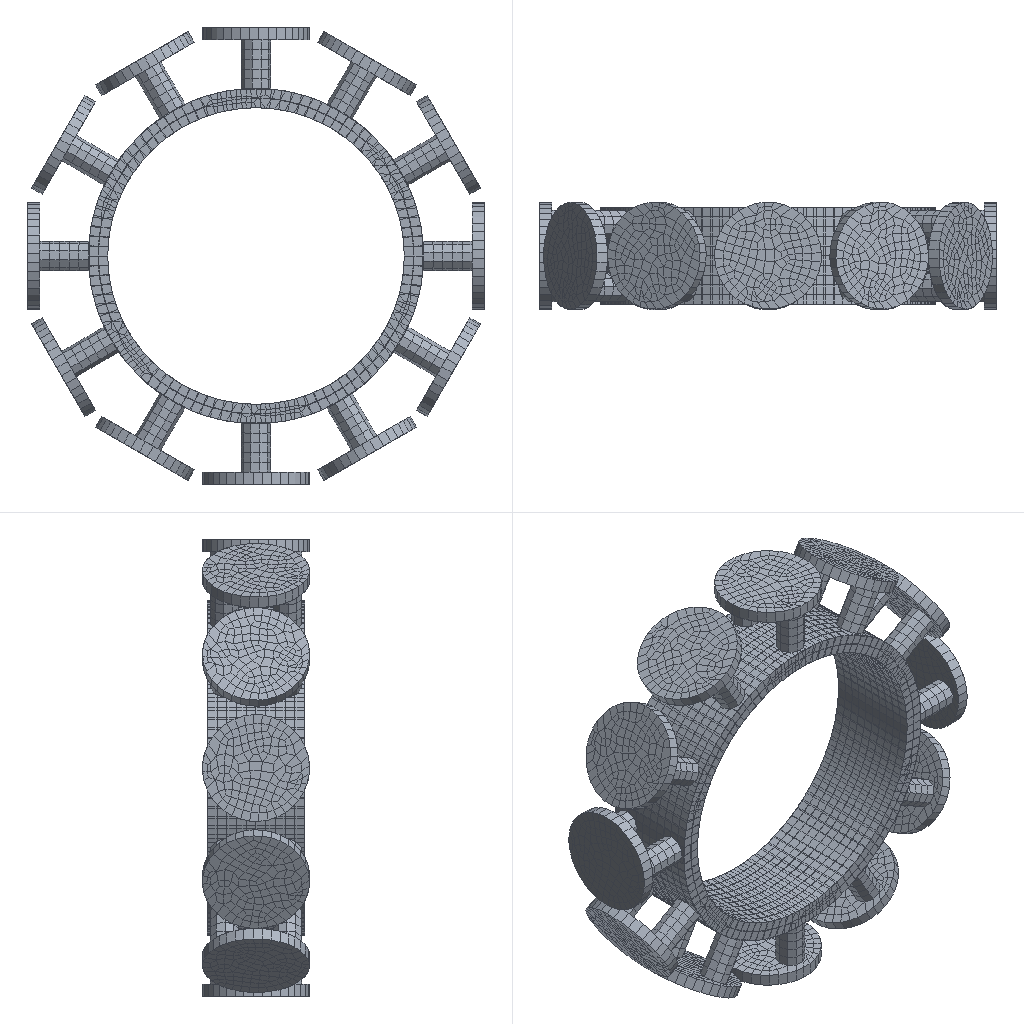Simulation study | abaqus
Set-up summary:
category,name,step,type,value,unit,region
solver,abaqus
solver,version,,,Abaqus/Standard 2020
units,not stated in the deck,,not stated
analysis,deck,,static,static
load_step,Step-1,Step-1,static
load_step,requested,,,1
mesh,nodes,,,21948
mesh,elements,,,16928
element_type,S4R,,shell,11811
element_type,C3D8R,,solid,5117
load,load commands in deck,,count,12
bc,support commands in deck,,count,5
material,CON,,in results
material,FRP,,in results
material,MATERIAL-3,,in results
check,setup vs results,,match,"per instance, exact: element labels, types and connectivity; labels of the nodes the elements use; coordinates of those nodes at SINGLE_PRECISION in 18 of 19 instance(s)"
Abaqus input file, long lists of numbers shortened:
*Heading
** Job name: Job-3 Model name: Model-1-Copy2-Copy
** Generated by: Abaqus/CAE 2020
*Preprint, echo=NO, model=NO, history=NO, contact=NO
**
** PARTS
**
*Part, name=con
*Node
      1,         610.,   1219.589,           0.
      2,         650.,   1219.589,           0.
** (916 more lines like these left out)
*Element, type=C3D8R
  1,  10,  11,  14,  13,   1,   2,   5,   4
  2,  11,  12,  15,  14,   2,   3,   6,   5
** (406 more lines like these left out)
*Nset, nset=Set-1, generate
   1,  918,    1
*Elset, elset=Set-1, generate
   1,  408,    1
** Section: con
*Solid Section, elset=Set-1, material=con
,
*End Part
**
*Part, name=frp
*Node
      1,   666.024,    1000.002,           0.
      2,   666.024,    1160.002,           0.
** (8318 more lines like these left out)
*Element, type=S4R
   1,   48,   41,    6,    1
   2,   41,   42,    7,    6
** (8318 more lines like these left out)
*Nset, nset=Set-3, generate
    1,  8320,     1
*Elset, elset=Set-3, generate
    1,  8320,     1
** Section: Section-1
*Shell Section, elset=Set-3, material=frp
7., 5
*End Part
**
*Part, name=gangban
*Node
      1,         610.,   1059.589,           0.
      2,         610.,   979.589,           0.
** (3081 more lines like these left out)
*Element, type=S4R
  1,    1,   13, 1241,  108
  2,   13,   14, 1242, 1241
** (3489 more lines like these left out)
*Nset, nset=Set-3, generate
    1,  3083,     1
*Elset, elset=Set-3, generate
    1,  3491,     1
** Section: Section-1
*Shell Section, elset=Set-3, material=frp
7., 5
*End Part
**
*Part, name=m1
*Node
      1,         890.,   1007.07,  -46.852
      2,   688.407,   1007.07,  -46.852
** (478 more lines like these left out)
*Element, type=C3D8R
 1, 434, 437, 435, 433, 114, 117, 115, 113
 2, 438, 434, 433, 436, 118, 114, 113, 116
** (239 more lines like these left out)
*Nset, nset=Set-1, generate
   1,  480,    1
*Elset, elset=Set-1, generate
   1,  241,    1
** Section: m
*Solid Section, elset=Set-1, material=Material-3
,
*End Part
**
*Part, name=m2
*Node
      1,   747.337,   1007.07,  -485.575
      2,   572.752,   1007.07,   -384.779
** (516 more lines like these left out)
*Element, type=C3D8R
 1, 119,  12,  11, 120, 453, 130, 129, 454
 2, 114,  10,   9, 121, 448, 128, 127, 455
** (273 more lines like these left out)
*Nset, nset=Set-3, generate
   1,  518,    1
*Elset, elset=Set-3, generate
   1,  275,    1
** Section: m
*Solid Section, elset=Set-3, material=Material-3
,
*End Part
**
*Part, name=m3
*Node
      1,   404.425,   1007.07,   -794.189
      2,   303.629,   1007.07,  -619.604
** (537 more lines like these left out)
*Element, type=C3D8R
 1, 119,  12,  11, 120, 462, 130, 129, 463
 2, 114,  10,   9, 121, 457, 128, 127, 464
** (291 more lines like these left out)
*Nset, nset=Set-1, generate
   1,  539,    1
*Elset, elset=Set-1, generate
   1,  293,    1
** Section: m
*Solid Section, elset=Set-1, material=Material-3
,
*End Part
**
*Part, name=m4
*Node
      1,  -46.852,   1007.07,        -890.
      2,  -46.852,   1007.07,  -688.407
** (478 more lines like these left out)
*Element, type=C3D8R
 1, 434, 437, 435, 433, 114, 117, 115, 113
 2, 438, 434, 433, 436, 118, 114, 113, 116
** (239 more lines like these left out)
*Nset, nset=Set-1, generate
   1,  480,    1
*Elset, elset=Set-1, generate
   1,  241,    1
** Section: m
*Solid Section, elset=Set-1, material=Material-3
,
*End Part
**
*Part, name=m5
*Node
      1,  -485.575,   1007.07,  -747.337
      2,   -384.779,   1007.07,  -572.752
** (487 more lines like these left out)
*Element, type=C3D8R
 1, 430, 123, 124, 434, 113,   8,   9, 117
 2, 432, 437, 433, 431, 115, 120, 116, 114
** (251 more lines like these left out)
*Nset, nset=Set-1, generate
   1,  489,    1
*Elset, elset=Set-1, generate
   1,  253,    1
** Section: m
*Solid Section, elset=Set-1, material=Material-3
,
*End Part
**
*Part, name=m6
*Node
      1,   -794.189,   1007.07,  -404.425
      2,  -619.604,   1007.07,  -303.629
** (466 more lines like these left out)
*Element, type=C3D8R
 1, 429, 118, 119, 120, 113,   8,   9,  10
 2, 125, 431, 430, 124,  15, 115, 114,  14
** (228 more lines like these left out)
*Nset, nset=Set-1, generate
   1,  468,    1
*Elset, elset=Set-1, generate
   1,  230,    1
** Section: m
*Solid Section, elset=Set-1, material=Material-3
,
*End Part
**
*Part, name=m7
*Node
      1,        -890.,   1007.07,   46.852
      2,  -688.407,   1007.07,   46.852
** (462 more lines like these left out)
*Element, type=C3D8R
 1, 118, 119, 427, 425,   8,   9, 115, 113
 2, 428, 426, 425, 427, 116, 114, 113, 115
** (226 more lines like these left out)
*Nset, nset=Set-1, generate
   1,  464,    1
*Elset, elset=Set-1, generate
   1,  228,    1
** Section: m
*Solid Section, elset=Set-1, material=Material-3
,
*End Part
**
*Part, name=m8
*Node
      1,  -747.337,   1007.07,   485.575
      2,  -572.752,   1007.07,    384.779
** (516 more lines like these left out)
*Element, type=C3D8R
 1, 119,  12,  11, 120, 453, 130, 129, 454
 2,  10,   9, 121, 114, 128, 127, 455, 448
** (273 more lines like these left out)
*Nset, nset=Set-1, generate
   1,  518,    1
*Elset, elset=Set-1, generate
   1,  275,    1
** Section: m
*Solid Section, elset=Set-1, material=Material-3
,
*End Part
**
*Part, name=m9
*Node
      1,  -404.425,   1007.07,    794.189
      2,  -303.629,   1007.07,   619.604
** (468 more lines like these left out)
*Element, type=C3D8R
 1, 423, 120, 121, 426, 113,   8,   9, 116
 2, 428, 426, 123, 124, 118, 116,  11,  12
** (234 more lines like these left out)
*Nset, nset=Set-1, generate
   1,  470,    1
*Elset, elset=Set-1, generate
   1,  236,    1
** Section: m
*Solid Section, elset=Set-1, material=Material-3
,
*End Part
**
*Part, name=m10
*Node
      1,   46.852,   1007.07,         890.
      2,   46.852,   1007.07,   688.407
** (541 more lines like these left out)
*Element, type=C3D8R
 1, 113, 123, 119, 120, 460, 470, 466, 467
 2, 114,  10,   9, 121, 461, 128, 127, 468
** (293 more lines like these left out)
*Nset, nset=Set-1, generate
   1,  543,    1
*Elset, elset=Set-1, generate
   1,  295,    1
** Section: m
*Solid Section, elset=Set-1, material=Material-3
,
*End Part
**
*Part, name=m11
*Node
      1,   485.575,   1007.07,   747.337
      2,    384.779,   1007.07,   572.752
** (516 more lines like these left out)
*Element, type=C3D8R
 1, 119,  12,  11, 120, 453, 130, 129, 454
 2, 114,  10,   9, 121, 448, 128, 127, 455
** (273 more lines like these left out)
*Nset, nset=Set-1, generate
   1,  518,    1
*Elset, elset=Set-1, generate
   1,  275,    1
** Section: m
*Solid Section, elset=Set-1, material=Material-3
,
*End Part
**
*Part, name=m12
*Node
      1,    794.189,   1007.07,   404.425
      2,   619.604,   1007.07,   303.629
** (466 more lines like these left out)
*Element, type=C3D8R
 1, 421, 120, 121, 424, 113,   8,   9, 116
 2, 426, 424, 123, 124, 118, 116,  11,  12
** (233 more lines like these left out)
*Nset, nset=Set-1, generate
   1,  468,    1
*Elset, elset=Set-1, generate
   1,  235,    1
** Section: m
*Solid Section, elset=Set-1, material=Material-3
,
*End Part
**
**
** ASSEMBLY
**
*Assembly, name=Assembly
**
*Instance, name=con-1, part=con
*End Instance
**
*Instance, name=frp-1, part=frp
*End Instance
**
*Instance, name=gangban-1, part=gangban
*End Instance
**
*Instance, name=con-1-lin-1-2, part=con
          0.,         -80.,           0.
*End Instance
**
*Instance, name=con-1-lin-1-3, part=con
          0.,        -160.,           0.
*End Instance
**
*Instance, name=con-1-lin-1-4, part=con
          0.,        -240.,           0.
*End Instance
**
*Instance, name=con-1-lin-1-5, part=con
          0.,        -320.,           0.
*End Instance
**
*Instance, name=m1-1, part=m1
*End Instance
**
*Instance, name=m2-1, part=m2
*End Instance
**
*Instance, name=m3-1, part=m3
*End Instance
**
*Instance, name=m4-1, part=m4
*End Instance
**
*Instance, name=m5-1, part=m5
*End Instance
**
*Instance, name=m6-1, part=m6
*End Instance
**
*Instance, name=m7-1, part=m7
*End Instance
**
*Instance, name=m8-1, part=m8
*End Instance
**
*Instance, name=m9-1, part=m9
*End Instance
**
*Instance, name=m10-1, part=m10
*End Instance
**
*Instance, name=m11-1, part=m11
*End Instance
**
*Instance, name=m12-1, part=m12
*End Instance
**
*Node
      1,         470.,   1099.589,   814.064
*Node
      2,   814.064,   1099.589,         470.
*Node
      3,         940.,   1099.589, 1.34711146e-14
*Node
      4,   814.064,   1099.589,        -470.
*Node
      5,         470.,   1099.589,  -814.064
*Node
      6, 7.10295131e-14,   1099.589,        -940.
*Node
      7,        -470.,   1099.589,  -814.064
*Node
      8,  -814.064,   1099.589,        -470.
*Node
      9,        -940.,   1099.589, -1.28587909e-13
*Node
     10,  -814.064,   1099.589,         470.
*Node
     11,        -470.,   1099.589,   814.064
*Node
     12, -1.86146319e-13,   1099.589,         940.
*Node
     13,           0.,   1059.589, -3.73517271e-14
*Nset, nset=Set-3, instance=con-1
   7,   8,   9,  16,  17,  18,  25,  26,  27,  34,  35,  36,  43,  44,  45,  52
  53,  54,  61,  62,  63,  70,  71,  72,  79,  80,  81,  88,  89,  90,  97,  98
** (18 more lines like these left out)
*Elset, elset=Set-3, instance=con-1
   3,   4,   7,   8,  11,  12,  15,  16,  19,  20,  23,  24,  27,  28,  31,  32
  35,  36,  39,  40,  43,  44,  47,  48,  51,  52,  55,  56,  59,  60,  63,  64
** (11 more lines like these left out)
*Nset, nset=Set-4, instance=m1-1
   4,   5,  34,  35,  36,  37,  38,  39,  40,  41,  42,  43,  44,  45,  46,  47
  48,  49,  50,  51,  52,  53,  54,  55,  56,  57,  58,  59,  60,  61,  62,  63
** (3 more lines like these left out)
*Nset, nset=Set-4, instance=m2-1
   4,   5,  34,  35,  36,  37,  38,  39,  40,  41,  42,  43,  44,  45,  46,  47
  48,  49,  50,  51,  52,  53,  54,  55,  56,  57,  58,  59,  60,  61,  62,  63
** (3 more lines like these left out)
*Nset, nset=Set-4, instance=m4-1
   4,   5,  34,  35,  36,  37,  38,  39,  40,  41,  42,  43,  44,  45,  46,  47
  48,  49,  50,  51,  52,  53,  54,  55,  56,  57,  58,  59,  60,  61,  62,  63
** (3 more lines like these left out)
*Nset, nset=Set-4, instance=m6-1
   4,   5,  34,  35,  36,  37,  38,  39,  40,  41,  42,  43,  44,  45,  46,  47
  48,  49,  50,  51,  52,  53,  54,  55,  56,  57,  58,  59,  60,  61,  62,  63
** (3 more lines like these left out)
*Nset, nset=Set-4, instance=m10-1
   4,   5,  34,  35,  36,  37,  38,  39,  40,  41,  42,  43,  44,  45,  46,  47
  48,  49,  50,  51,  52,  53,  54,  55,  56,  57,  58,  59,  60,  61,  62,  63
** (3 more lines like these left out)
*Nset, nset=Set-4, instance=m8-1
   4,   5,  34,  35,  36,  37,  38,  39,  40,  41,  42,  43,  44,  45,  46,  47
  48,  49,  50,  51,  52,  53,  54,  55,  56,  57,  58,  59,  60,  61,  62,  63
** (3 more lines like these left out)
*Nset, nset=Set-4, instance=m12-1
   4,   5,  34,  35,  36,  37,  38,  39,  40,  41,  42,  43,  44,  45,  46,  47
  48,  49,  50,  51,  52,  53,  54,  55,  56,  57,  58,  59,  60,  61,  62,  63
** (3 more lines like these left out)
*Nset, nset=Set-4, instance=m3-1
   4,   5,  34,  35,  36,  37,  38,  39,  40,  41,  42,  43,  44,  45,  46,  47
  48,  49,  50,  51,  52,  53,  54,  55,  56,  57,  58,  59,  60,  61,  62,  63
** (3 more lines like these left out)
*Nset, nset=Set-4, instance=m7-1
   4,   5,  34,  35,  36,  37,  38,  39,  40,  41,  42,  43,  44,  45,  46,  47
  48,  49,  50,  51,  52,  53,  54,  55,  56,  57,  58,  59,  60,  61,  62,  63
** (3 more lines like these left out)
*Nset, nset=Set-4, instance=m11-1
   4,   5,  34,  35,  36,  37,  38,  39,  40,  41,  42,  43,  44,  45,  46,  47
  48,  49,  50,  51,  52,  53,  54,  55,  56,  57,  58,  59,  60,  61,  62,  63
** (3 more lines like these left out)
*Nset, nset=Set-4, instance=m5-1
   4,   5,  34,  35,  36,  37,  38,  39,  40,  41,  42,  43,  44,  45,  46,  47
  48,  49,  50,  51,  52,  53,  54,  55,  56,  57,  58,  59,  60,  61,  62,  63
** (3 more lines like these left out)
*Nset, nset=Set-4, instance=m9-1
   4,   5,  34,  35,  36,  37,  38,  39,  40,  41,  42,  43,  44,  45,  46,  47
  48,  49,  50,  51,  52,  53,  54,  55,  56,  57,  58,  59,  60,  61,  62,  63
** (3 more lines like these left out)
*Elset, elset=Set-4, instance=m1-1
  77,  80,  82,  83,  84,  86,  88,  90,  91,  92,  98,  99, 100, 104, 105, 106
 107, 109, 111, 112, 113, 116, 118, 122, 129, 130, 131, 132, 133, 134, 136, 137
** (1 more lines like these left out)
*Elset, elset=Set-4, instance=m2-1
 101, 106, 107, 108, 109, 110, 111, 112, 113, 115, 117, 122, 123, 130, 131, 132
 133, 134, 138, 141, 143, 147, 153, 154, 156, 157, 158, 159, 160, 161, 164, 165
** (1 more lines like these left out)
*Elset, elset=Set-4, instance=m4-1
  77,  80,  82,  83,  84,  87,  89,  91,  92,  93,  99, 100, 101, 104, 105, 106
 107, 109, 111, 112, 113, 116, 117, 121, 129, 130, 131, 132, 133, 134, 136, 137
** (1 more lines like these left out)
*Elset, elset=Set-4, instance=m6-1
  52,  53,  61,  62,  66,  67,  68,  70,  71,  72,  73,  74,  76,  80,  84,  88
  89,  92,  93,  94,  97, 101, 107, 112, 113, 114, 117, 118, 119, 121, 122, 124
** (1 more lines like these left out)
*Elset, elset=Set-4, instance=m10-1
 103, 111, 112, 114, 115, 116, 118, 120, 123, 124, 126, 131, 133, 137, 138, 139
 140, 142, 145, 148, 150, 153, 160, 161, 162, 163, 164, 165, 166, 167, 168, 170
** (1 more lines like these left out)
*Elset, elset=Set-4, instance=m8-1
 100, 105, 106, 107, 108, 109, 110, 111, 112, 113, 115, 120, 121, 122, 130, 131
 133, 134, 138, 142, 145, 153, 154, 155, 156, 157, 158, 159, 161, 162, 165, 166
** (1 more lines like these left out)
*Elset, elset=Set-4, instance=m12-1
  62,  63,  71,  75,  76,  77,  79,  80,  81,  82,  83,  85,  89,  91,  94,  97
  98, 101, 102, 103, 106, 110, 115, 122, 123, 124, 125, 126, 129, 130, 134, 135
** (1 more lines like these left out)
*Elset, elset=Set-4, instance=m3-1
  95,  96, 104, 109, 110, 111, 113, 114, 115, 116, 118, 123, 124, 127, 131, 132
 135, 136, 138, 141, 145, 149, 153, 158, 159, 161, 162, 163, 165, 166, 168, 169
** (1 more lines like these left out)
*Elset, elset=Set-4, instance=m7-1
  67,  70,  72,  73,  74,  77,  79,  81,  82,  83,  89,  90,  91,  94,  95,  96
  97,  99, 100, 101, 102, 105, 106, 111, 118, 119, 120, 122, 123, 124, 126, 127
** (1 more lines like these left out)
*Elset, elset=Set-4, instance=m11-1
 101, 106, 107, 109, 110, 111, 112, 113, 115, 117, 122, 123, 124, 131, 132, 133
 134, 138, 141, 145, 147, 152, 153, 154, 155, 157, 159, 160, 161, 162, 165, 166
** (1 more lines like these left out)
*Elset, elset=Set-4, instance=m5-1
  86,  91,  92,  93,  94,  96,  97,  98, 100, 102, 106, 115, 116, 117, 118, 119
 121, 124, 126, 133, 137, 138, 140, 141, 142, 143, 144, 145, 146, 147, 151, 152
** (1 more lines like these left out)
*Elset, elset=Set-4, instance=m9-1
  62,  63,  71,  75,  76,  77,  78,  80,  81,  82,  83,  85,  87,  91,  93,  99
 100, 103, 104, 105, 108, 112, 117, 120, 124, 125, 126, 127, 130, 131, 135, 136
** (1 more lines like these left out)
*Nset, nset=Set-30
 13,
*Nset, nset=b_Set-5, instance=m11-1, generate
   1,  518,    1
*Elset, elset=b_Set-5, instance=m11-1, generate
   1,  275,    1
*Nset, nset=b_Set-7, instance=m12-1, generate
   1,  468,    1
*Elset, elset=b_Set-7, instance=m12-1, generate
   1,  235,    1
*Nset, nset=b_Set-9, instance=m1-1, generate
   1,  480,    1
*Elset, elset=b_Set-9, instance=m1-1, generate
   1,  241,    1
*Nset, nset=b_Set-11, instance=m2-1, generate
   1,  518,    1
*Elset, elset=b_Set-11, instance=m2-1, generate
   1,  275,    1
*Nset, nset=b_Set-13, instance=m3-1, generate
   1,  539,    1
*Elset, elset=b_Set-13, instance=m3-1, generate
   1,  293,    1
*Nset, nset=b_Set-15, instance=m4-1, generate
   1,  480,    1
*Elset, elset=b_Set-15, instance=m4-1, generate
   1,  241,    1
*Nset, nset=b_Set-17, instance=m5-1, generate
   1,  489,    1
*Elset, elset=b_Set-17, instance=m5-1, generate
   1,  253,    1
*Nset, nset=b_Set-19, instance=m6-1, generate
   1,  468,    1
*Elset, elset=b_Set-19, instance=m6-1, generate
   1,  230,    1
*Nset, nset=b_Set-21, instance=m7-1, generate
   1,  464,    1
*Elset, elset=b_Set-21, instance=m7-1, generate
   1,  228,    1
*Nset, nset=b_Set-23, instance=m8-1, generate
   1,  518,    1
*Elset, elset=b_Set-23, instance=m8-1, generate
   1,  275,    1
*Nset, nset=b_Set-25, instance=m9-1, generate
   1,  470,    1
*Elset, elset=b_Set-25, instance=m9-1, generate
   1,  236,    1
*Nset, nset=b_Set-27, instance=m10-1, generate
   1,  543,    1
*Elset, elset=b_Set-27, instance=m10-1, generate
   1,  295,    1
*Nset, nset=m_Set-1, instance=frp-1, generate
    1,  8320,     1
*Elset, elset=m_Set-1, instance=frp-1, generate
    1,  8320,     1
*Nset, nset=m_Set-29
 13,
*Nset, nset=s_Set-1, instance=con-1, generate
   1,  918,    1
*Nset, nset=s_Set-1, instance=con-1-lin-1-2, generate
   1,  918,    1
*Nset, nset=s_Set-1, instance=con-1-lin-1-3, generate
   1,  918,    1
*Nset, nset=s_Set-1, instance=con-1-lin-1-5, generate
   1,  918,    1
*Nset, nset=s_Set-1, instance=con-1-lin-1-4, generate
   1,  918,    1
*Elset, elset=s_Set-1, instance=con-1, generate
   1,  408,    1
*Elset, elset=s_Set-1, instance=con-1-lin-1-2, generate
   1,  408,    1
*Elset, elset=s_Set-1, instance=con-1-lin-1-3, generate
   1,  408,    1
*Elset, elset=s_Set-1, instance=con-1-lin-1-5, generate
   1,  408,    1
*Elset, elset=s_Set-1, instance=con-1-lin-1-4, generate
   1,  408,    1
*Nset, nset=_PickedSet98, internal
 1,
*Nset, nset=_PickedSet100, internal
 2,
*Nset, nset=_PickedSet102, internal
 3,
*Nset, nset=_PickedSet104, internal
 4,
*Nset, nset=_PickedSet106, internal
 5,
*Nset, nset=_PickedSet108, internal
 6,
*Nset, nset=_PickedSet110, internal
 7,
*Nset, nset=_PickedSet112, internal
 8,
*Nset, nset=_PickedSet114, internal
 9,
*Nset, nset=_PickedSet116, internal
 10,
*Nset, nset=_PickedSet118, internal
 11,
*Nset, nset=_PickedSet120, internal
 12,
*Elset, elset=_Surf-1_S1, internal, instance=m10-1, generate
  81,  214,    1
*Elset, elset=_Surf-1_S2, internal, instance=m10-1, generate
 215,  230,    1
*Surface, type=ELEMENT, name=Surf-1
_Surf-1_S1, S1
_Surf-1_S2, S2
*Elset, elset=_Surf-2_S2, internal, instance=m9-1
  51,  52,  53,  54,  55,  56,  57,  58,  59,  60, 177, 178, 179, 180, 181, 182
 183, 184, 185, 186
*Elset, elset=_Surf-2_S1, internal, instance=m9-1, generate
  61,  176,    1
*Surface, type=ELEMENT, name=Surf-2
_Surf-2_S2, S2
_Surf-2_S1, S1
*Elset, elset=_Surf-3_S1, internal, instance=m8-1, generate
  81,  209,    1
*Elset, elset=_Surf-3_S2, internal, instance=m8-1, generate
 210,  225,    1
*Surface, type=ELEMENT, name=Surf-3
_Surf-3_S1, S1
_Surf-3_S2, S2
*Elset, elset=_Surf-4_S2, internal, instance=m7-1
  41,  42,  43,  44,  45,  46,  47,  48,  49,  50, 171, 172, 173, 174, 175, 176
 177, 178
*Elset, elset=_Surf-4_S1, internal, instance=m7-1, generate
  51,  170,    1
*Surface, type=ELEMENT, name=Surf-4
_Surf-4_S2, S2
_Surf-4_S1, S1
*Elset, elset=_Surf-5_S2, internal, instance=m6-1
  41,  42,  43,  44,  45,  46,  47,  48,  49,  50, 173, 174, 175, 176, 177, 178
 179, 180
*Elset, elset=_Surf-5_S1, internal, instance=m6-1, generate
  51,  172,    1
*Surface, type=ELEMENT, name=Surf-5
_Surf-5_S2, S2
_Surf-5_S1, S1
*Elset, elset=_Surf-6_S2, internal, instance=m5-1
  66,  67,  68,  69,  70,  71,  72,  73,  74,  75, 191, 192, 193, 194, 195, 196
 197, 198, 199, 200, 201, 202, 203
*Elset, elset=_Surf-6_S1, internal, instance=m5-1, generate
  76,  190,    1
*Surface, type=ELEMENT, name=Surf-6
_Surf-6_S2, S2
_Surf-6_S1, S1
*Elset, elset=_Surf-7_S2, internal, instance=m4-1
  51,  52,  53,  54,  55,  56,  57,  58,  59,  60, 182, 183, 184, 185, 186, 187
 188, 189, 190, 191
*Elset, elset=_Surf-7_S1, internal, instance=m4-1, generate
  61,  181,    1
*Surface, type=ELEMENT, name=Surf-7
_Surf-7_S2, S2
_Surf-7_S1, S1
*Elset, elset=_Surf-8_S1, internal, instance=m3-1, generate
  81,  212,    1
*Elset, elset=_Surf-8_S2, internal, instance=m3-1, generate
 213,  228,    1
*Surface, type=ELEMENT, name=Surf-8
_Surf-8_S1, S1
_Surf-8_S2, S2
*Elset, elset=_Surf-9_S1, internal, instance=m2-1, generate
  81,  209,    1
*Elset, elset=_Surf-9_S2, internal, instance=m2-1, generate
 210,  225,    1
*Surface, type=ELEMENT, name=Surf-9
_Surf-9_S1, S1
_Surf-9_S2, S2
*Elset, elset=_Surf-10_S2, internal, instance=m1-1
  51,  52,  53,  54,  55,  56,  57,  58,  59,  60, 182, 183, 184, 185, 186, 187
 188, 189, 190, 191
*Elset, elset=_Surf-10_S1, internal, instance=m1-1, generate
  61,  181,    1
*Surface, type=ELEMENT, name=Surf-10
_Surf-10_S2, S2
_Surf-10_S1, S1
*Elset, elset=_Surf-11_S2, internal, instance=m12-1
  51,  52,  53,  54,  55,  56,  57,  58,  59,  60, 176, 177, 178, 179, 180, 181
 182, 183, 184, 185
*Elset, elset=_Surf-11_S1, internal, instance=m12-1, generate
  61,  175,    1
*Surface, type=ELEMENT, name=Surf-11
_Surf-11_S2, S2
_Surf-11_S1, S1
*Elset, elset=_Surf-12_S1, internal, instance=m11-1, generate
  81,  209,    1
*Elset, elset=_Surf-12_S2, internal, instance=m11-1, generate
 210,  225,    1
*Surface, type=ELEMENT, name=Surf-12
_Surf-12_S1, S1
_Surf-12_S2, S2
*Elset, elset=_m_Surf-15_S3, internal, instance=con-1
   1,   2,   5,   6,   9,  10,  13,  14,  17,  18,  21,  22,  25,  26,  29,  30
  33,  34,  37,  38,  41,  42,  45,  46,  49,  50,  53,  54,  57,  58,  61,  62
** (11 more lines like these left out)
*Elset, elset=_m_Surf-15_S3, internal, instance=con-1-lin-1-2
   1,   2,   5,   6,   9,  10,  13,  14,  17,  18,  21,  22,  25,  26,  29,  30
  33,  34,  37,  38,  41,  42,  45,  46,  49,  50,  53,  54,  57,  58,  61,  62
** (11 more lines like these left out)
*Elset, elset=_m_Surf-15_S3, internal, instance=con-1-lin-1-3
   1,   2,   5,   6,   9,  10,  13,  14,  17,  18,  21,  22,  25,  26,  29,  30
  33,  34,  37,  38,  41,  42,  45,  46,  49,  50,  53,  54,  57,  58,  61,  62
** (11 more lines like these left out)
*Elset, elset=_m_Surf-15_S3, internal, instance=con-1-lin-1-5
   1,   2,   5,   6,   9,  10,  13,  14,  17,  18,  21,  22,  25,  26,  29,  30
  33,  34,  37,  38,  41,  42,  45,  46,  49,  50,  53,  54,  57,  58,  61,  62
** (11 more lines like these left out)
*Elset, elset=_m_Surf-15_S3, internal, instance=con-1-lin-1-4
   1,   2,   5,   6,   9,  10,  13,  14,  17,  18,  21,  22,  25,  26,  29,  30
  33,  34,  37,  38,  41,  42,  45,  46,  49,  50,  53,  54,  57,  58,  61,  62
** (11 more lines like these left out)
*Elset, elset=_m_Surf-15_S6, internal, instance=con-1, generate
   1,  407,    2
*Elset, elset=_m_Surf-15_S6, internal, instance=con-1-lin-1-2, generate
   1,  407,    2
*Elset, elset=_m_Surf-15_S6, internal, instance=con-1-lin-1-3, generate
   1,  407,    2
*Elset, elset=_m_Surf-15_S6, internal, instance=con-1-lin-1-5, generate
   1,  407,    2
*Elset, elset=_m_Surf-15_S6, internal, instance=con-1-lin-1-4, generate
   1,  407,    2
*Elset, elset=_m_Surf-15_S5, internal, instance=con-1
   3,   4,   7,   8,  11,  12,  15,  16,  19,  20,  23,  24,  27,  28,  31,  32
  35,  36,  39,  40,  43,  44,  47,  48,  51,  52,  55,  56,  59,  60,  63,  64
** (11 more lines like these left out)
*Elset, elset=_m_Surf-15_S5, internal, instance=con-1-lin-1-2
   3,   4,   7,   8,  11,  12,  15,  16,  19,  20,  23,  24,  27,  28,  31,  32
  35,  36,  39,  40,  43,  44,  47,  48,  51,  52,  55,  56,  59,  60,  63,  64
** (11 more lines like these left out)
*Elset, elset=_m_Surf-15_S5, internal, instance=con-1-lin-1-3
   3,   4,   7,   8,  11,  12,  15,  16,  19,  20,  23,  24,  27,  28,  31,  32
  35,  36,  39,  40,  43,  44,  47,  48,  51,  52,  55,  56,  59,  60,  63,  64
** (11 more lines like these left out)
*Elset, elset=_m_Surf-15_S5, internal, instance=con-1-lin-1-5
   3,   4,   7,   8,  11,  12,  15,  16,  19,  20,  23,  24,  27,  28,  31,  32
  35,  36,  39,  40,  43,  44,  47,  48,  51,  52,  55,  56,  59,  60,  63,  64
** (11 more lines like these left out)
*Elset, elset=_m_Surf-15_S5, internal, instance=con-1-lin-1-4
   3,   4,   7,   8,  11,  12,  15,  16,  19,  20,  23,  24,  27,  28,  31,  32
  35,  36,  39,  40,  43,  44,  47,  48,  51,  52,  55,  56,  59,  60,  63,  64
** (11 more lines like these left out)
*Elset, elset=_m_Surf-15_S4, internal, instance=con-1, generate
   2,  408,    2
*Elset, elset=_m_Surf-15_S4, internal, instance=con-1-lin-1-2, generate
   2,  408,    2
*Elset, elset=_m_Surf-15_S4, internal, instance=con-1-lin-1-3, generate
   2,  408,    2
*Elset, elset=_m_Surf-15_S4, internal, instance=con-1-lin-1-5, generate
   2,  408,    2
*Elset, elset=_m_Surf-15_S4, internal, instance=con-1-lin-1-4, generate
   2,  408,    2
*Surface, type=ELEMENT, name=m_Surf-15
_m_Surf-15_S3, S3
_m_Surf-15_S6, S6
_m_Surf-15_S4, S4
_m_Surf-15_S5, S5
*Elset, elset=_m_Surf-17_SPOS, internal, instance=gangban-1
  193,  194,  195,  196,  197,  198,  199,  200,  201,  202,  203,  204,  205,  206,  207,  208
  209,  210,  211,  212,  213,  214,  215,  216,  217,  218,  219,  220,  221,  222,  223,  224
** (66 more lines like these left out)
*Surface, type=ELEMENT, name=m_Surf-17
_m_Surf-17_SPOS, SPOS
*Elset, elset=_s_Surf-14_SPOS, internal, instance=gangban-1, generate
 3017,  3491,     1
*Surface, type=ELEMENT, name=s_Surf-14
_s_Surf-14_SPOS, SPOS
*Elset, elset=_s_Surf-15_SNEG, internal, instance=gangban-1, generate
    1,  3491,     1
*Surface, type=ELEMENT, name=s_Surf-15
_s_Surf-15_SNEG, SNEG
*Elset, elset=_s_Surf-17_S2, internal, instance=m1-1, generate
 232,  241,    1
*Elset, elset=_s_Surf-17_S2, internal, instance=m2-1
  65,  66,  67,  68,  69,  70,  71,  72,  73,  74,  75,  76,  77,  78,  79,  80
 266, 267, 268, 269, 270, 271, 272, 273, 274, 275
*Elset, elset=_s_Surf-17_S2, internal, instance=m4-1, generate
 232,  241,    1
*Elset, elset=_s_Surf-17_S2, internal, instance=m6-1, generate
 221,  230,    1
*Elset, elset=_s_Surf-17_S2, internal, instance=m10-1
  65,  66,  67,  68,  69,  70,  71,  72,  73,  74,  75,  76,  77,  78,  79,  80
 283, 284, 285, 286, 287, 288, 289, 290, 291, 292, 293, 294, 295
*Elset, elset=_s_Surf-17_S2, internal, instance=m8-1
  65,  66,  67,  68,  69,  70,  71,  72,  73,  74,  75,  76,  77,  78,  79,  80
 266, 267, 268, 269, 270, 271, 272, 273, 274, 275
*Elset, elset=_s_Surf-17_S2, internal, instance=m12-1, generate
 226,  235,    1
*Elset, elset=_s_Surf-17_S2, internal, instance=m3-1
  65,  66,  67,  68,  69,  70,  71,  72,  73,  74,  75,  76,  77,  78,  79,  80
 281, 282, 283, 284, 285, 286, 287, 288, 289, 290, 291, 292, 293
*Elset, elset=_s_Surf-17_S2, internal, instance=m7-1, generate
 219,  228,    1
*Elset, elset=_s_Surf-17_S2, internal, instance=m11-1
  65,  66,  67,  68,  69,  70,  71,  72,  73,  74,  75,  76,  77,  78,  79,  80
 266, 267, 268, 269, 270, 271, 272, 273, 274, 275
*Elset, elset=_s_Surf-17_S2, internal, instance=m5-1, generate
 244,  253,    1
*Elset, elset=_s_Surf-17_S2, internal, instance=m9-1, generate
 227,  236,    1
*Elset, elset=_s_Surf-17_S1, internal, instance=m1-1, generate
 41,  50,   1
*Elset, elset=_s_Surf-17_S1, internal, instance=m4-1, generate
 41,  50,   1
*Elset, elset=_s_Surf-17_S1, internal, instance=m6-1, generate
 33,  40,   1
*Elset, elset=_s_Surf-17_S1, internal, instance=m12-1, generate
 41,  50,   1
*Elset, elset=_s_Surf-17_S1, internal, instance=m7-1, generate
 33,  40,   1
*Elset, elset=_s_Surf-17_S1, internal, instance=m5-1, generate
 53,  65,   1
*Elset, elset=_s_Surf-17_S1, internal, instance=m9-1, generate
 41,  50,   1
*Surface, type=ELEMENT, name=s_Surf-17
_s_Surf-17_S2, S2
_s_Surf-17_S1, S1
*Elset, elset=_shuchu_SPOS, internal, instance=gangban-1
  193,  194,  195,  196,  197,  198,  199,  200,  201,  202,  203,  204,  205,  206,  207,  208
  209,  210,  211,  212,  213,  214,  215,  216,  217,  218,  219,  220,  221,  222,  223,  224
** (66 more lines like these left out)
*Surface, type=ELEMENT, name=shuchu
_shuchu_SPOS, SPOS
** Constraint: Constraint-1
*Embedded Element, host elset=s_Set-1
m_Set-1
** Constraint: Constraint-2
*Rigid Body, ref node=_PickedSet98, elset=b_Set-5
** Constraint: Constraint-3
*Rigid Body, ref node=_PickedSet100, elset=b_Set-7
** Constraint: Constraint-4
*Rigid Body, ref node=_PickedSet102, elset=b_Set-9
** Constraint: Constraint-5
*Rigid Body, ref node=_PickedSet104, elset=b_Set-11
** Constraint: Constraint-6
*Rigid Body, ref node=_PickedSet106, elset=b_Set-13
** Constraint: Constraint-7
*Rigid Body, ref node=_PickedSet108, elset=b_Set-15
** Constraint: Constraint-8
*Rigid Body, ref node=_PickedSet110, elset=b_Set-17
** Constraint: Constraint-9
*Rigid Body, ref node=_PickedSet112, elset=b_Set-19
** Constraint: Constraint-10
*Rigid Body, ref node=_PickedSet114, elset=b_Set-21
** Constraint: Constraint-11
*Rigid Body, ref node=_PickedSet116, elset=b_Set-23
** Constraint: Constraint-12
*Rigid Body, ref node=_PickedSet118, elset=b_Set-25
** Constraint: Constraint-13
*Rigid Body, ref node=_PickedSet120, elset=b_Set-27
** Constraint: Constraint-15
*Tie, name=Constraint-15, adjust=yes
m_Surf-15, s_Surf-15
** Constraint: Constraint-SHUCHU
*Coupling, constraint name=Constraint-SHUCHU, ref node=m_Set-29, surface=s_Surf-14
*Kinematic
*End Assembly
*Amplitude, name=Amp-1
             0.,              0.,              1.,              1.
**
** MATERIALS
**
*Material, name=Material-3
*Density
 7.8e-09,
*Elastic
180000., 0.3
*Plastic
147.,0.
*Material, name=con
*Density
 2.2e-09,
*Elastic
35900., 0.22
*Plastic
30.,0.
*Material, name=frp
*Density
 1.5e-09,
*Elastic, type=ENGINEERING CONSTANTS
11810.,11200.,11810.,  0.24,  0.23,  0.23, 7800., 8900.
 8900.,
**
** INTERACTION PROPERTIES
**
*Surface Interaction, name=IntProp-1
1.,
*Friction, slip tolerance=0.005
 0.2,
*Surface Behavior, pressure-overclosure=HARD
**
** INTERACTIONS
**
** Interaction: Int-2
*Contact Pair, interaction=IntProp-1, type=SURFACE TO SURFACE, adjust=1.
m_Surf-17, s_Surf-17
** ----------------------------------------------------------------
**
** STEP: Step-1
**
*Step, name=Step-1, nlgeom=YES, inc=1000
*Static, stabilize=0.0002, allsdtol=0.05, continue=NO
0.01, 1., 1e-05, 1.
**
** BOUNDARY CONDITIONS
**
** Name: BC-2 Type: 位移/转角
*Boundary
Set-4, 2, 2
Set-4, 4, 4
Set-4, 5, 5
Set-4, 6, 6
** Name: BC-3 Type: 对称/反对称/完全固定
*Boundary
Set-30, ENCASTRE
**
** LOADS
**
** Name: Load-1   Type: Pressure
*Dsload, amplitude=Amp-1
Surf-1, P, 200.
** Name: Load-2   Type: Pressure
*Dsload, amplitude=Amp-1
Surf-2, P, 210.
** Name: Load-3   Type: Pressure
*Dsload, amplitude=Amp-1
Surf-3, P, 240.
** Name: Load-4   Type: Pressure
*Dsload, amplitude=Amp-1
Surf-4, P, 190.
** Name: Load-5   Type: Pressure
*Dsload, amplitude=Amp-1
Surf-5, P, 213.
** Name: Load-6   Type: Pressure
*Dsload, amplitude=Amp-1
Surf-6, P, 207.
** Name: Load-7   Type: Pressure
*Dsload, amplitude=Amp-1
Surf-7, P, 220.
** Name: Load-8   Type: Pressure
*Dsload, amplitude=Amp-1
Surf-8, P, 223.
** Name: Load-9   Type: Pressure
*Dsload, amplitude=Amp-1
Surf-9, P, 230.
** Name: Load-10   Type: Pressure
*Dsload, amplitude=Amp-1
Surf-10, P, 224.
** Name: Load-11   Type: Pressure
*Dsload, amplitude=Amp-1
Surf-11, P, 218.
** Name: Load-12   Type: Pressure
*Dsload, amplitude=Amp-1
Surf-12, P, 211.
**
** OUTPUT REQUESTS
**
*Restart, write, number interval=1, time marks=NO
**
** FIELD OUTPUT: F-Output-1
**
*Output, field
*Node Output
CF, RF, RM, RT, U, V
*Element Output, directions=YES
E, LE, MISES, MISESMAX, MISESONLY, PE, PEEQ, S, SF, SSAVG
*Contact Output
CDISP, CSTRESS
**
** HISTORY OUTPUT: H-Output-1
**
*Output, history
*Node Output, nset=Set-30
RF1, RF3, U1, U3
*End Step
Results summary:
result,step,,partial,increments=40 time=0.4247/1.0
result,analysis,,,static
result,last_loadstep,,,1
result,primary field,,,"U, UR"
result,reaction total,,FX,2455791.0,model units
result,reaction total,,FY,-3411.58,model units
result,reaction total,,FZ,-1297583.75,model units